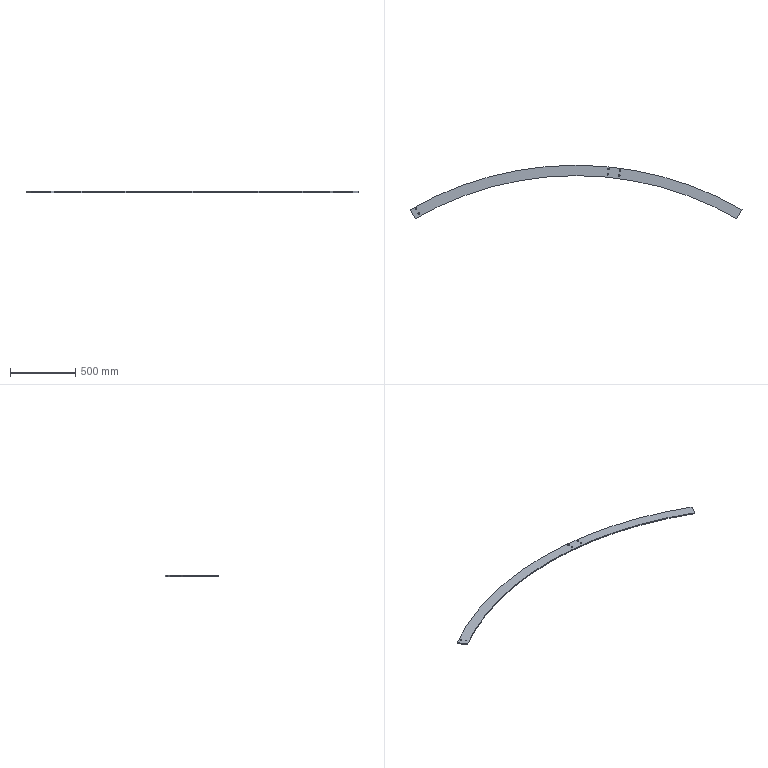Part | SolidWorks | features Extrusion 1, HoleWzd 1 | 1 solid | 18 faces | box 2550 x 410.917 x 8 mm | volume 1676789 mm3 | cylinder 14 | plane 4 | commonest cylinder face diameters 12 x12 4940 x1 5100 x1
STEP:
#1=CARTESIAN_POINT('',(-1221.329,76.713,0.));
#2=VERTEX_POINT('',#1);
#3=CARTESIAN_POINT('',(-1233.329,76.713,0.));
#4=VERTEX_POINT('',#3);
#5=CARTESIAN_POINT('',(-1227.329,76.713,0.));
#6=DIRECTION('',(0.,0.,-1.));
#7=DIRECTION('',(-1.,0.,0.));
#8=AXIS2_PLACEMENT_3D('',#5,#6,#7);
#9=CIRCLE('',#8,6.);
#10=EDGE_CURVE('',#2,#4,#9,.T.);
#11=ORIENTED_EDGE('',*,*,#10,.T.);
#12=CARTESIAN_POINT('',(-1233.329,76.713,8.));
#13=VERTEX_POINT('',#12);
#14=CARTESIAN_POINT('',(-1233.329,76.713,8.));
#15=DIRECTION('',(0.,0.,1.));
#16=VECTOR('',#15,1000.);
#17=LINE('',#14,#16);
#18=EDGE_CURVE('',#4,#13,#17,.T.);
#19=ORIENTED_EDGE('',*,*,#18,.T.);
#20=CARTESIAN_POINT('',(-1221.329,76.713,8.));
#21=VERTEX_POINT('',#20);
#22=CARTESIAN_POINT('',(-1227.329,76.713,8.));
#23=DIRECTION('',(0.,0.,1.));
#24=DIRECTION('',(1.,0.,0.));
#25=AXIS2_PLACEMENT_3D('',#22,#23,#24);
#26=CIRCLE('',#25,6.);
#27=EDGE_CURVE('',#13,#21,#26,.T.);
#28=ORIENTED_EDGE('',*,*,#27,.T.);
#29=CARTESIAN_POINT('',(-1221.329,76.713,8.));
#30=DIRECTION('',(0.,0.,1.));
#31=VECTOR('',#30,1000.);
#32=LINE('',#29,#31);
#33=EDGE_CURVE('',#2,#21,#32,.T.);
#34=ORIENTED_EDGE('',*,*,#33,.F.);
#35=EDGE_LOOP('',(#11,#19,#28,#34));
#36=FACE_OUTER_BOUND('',#35,.T.);
#37=CARTESIAN_POINT('',(-1227.329,76.713,8.));
#38=DIRECTION('',(0.,0.,1.));
#39=DIRECTION('',(1.,0.,0.));
#40=AXIS2_PLACEMENT_3D('',#37,#38,#39);
#41=CYLINDRICAL_SURFACE('',#40,6.);
#42=ADVANCED_FACE('',(#36),#41,.F.);
#43=CARTESIAN_POINT('',(-1201.948,41.723,0.));
#44=VERTEX_POINT('',#43);
#45=CARTESIAN_POINT('',(-1213.948,41.723,0.));
#46=VERTEX_POINT('',#45);
#47=CARTESIAN_POINT('',(-1207.948,41.723,0.));
#48=DIRECTION('',(0.,0.,-1.));
#49=DIRECTION('',(-1.,0.,0.));
#50=AXIS2_PLACEMENT_3D('',#47,#48,#49);
#51=CIRCLE('',#50,6.);
#52=EDGE_CURVE('',#44,#46,#51,.T.);
#53=ORIENTED_EDGE('',*,*,#52,.T.);
#54=CARTESIAN_POINT('',(-1213.948,41.723,8.));
#55=VERTEX_POINT('',#54);
#56=CARTESIAN_POINT('',(-1213.948,41.723,8.));
#57=DIRECTION('',(0.,0.,1.));
#58=VECTOR('',#57,1000.);
#59=LINE('',#56,#58);
#60=EDGE_CURVE('',#46,#55,#59,.T.);
#61=ORIENTED_EDGE('',*,*,#60,.T.);
#62=CARTESIAN_POINT('',(-1201.948,41.723,8.));
#63=VERTEX_POINT('',#62);
#64=CARTESIAN_POINT('',(-1207.948,41.723,8.));
#65=DIRECTION('',(0.,0.,1.));
#66=DIRECTION('',(1.,0.,0.));
#67=AXIS2_PLACEMENT_3D('',#64,#65,#66);
#68=CIRCLE('',#67,6.);
#69=EDGE_CURVE('',#55,#63,#68,.T.);
#70=ORIENTED_EDGE('',*,*,#69,.T.);
#71=CARTESIAN_POINT('',(-1201.948,41.723,8.));
#72=DIRECTION('',(0.,0.,1.));
#73=VECTOR('',#72,1000.);
#74=LINE('',#71,#73);
#75=EDGE_CURVE('',#44,#63,#74,.T.);
#76=ORIENTED_EDGE('',*,*,#75,.F.);
#77=EDGE_LOOP('',(#53,#61,#70,#76));
#78=FACE_OUTER_BOUND('',#77,.T.);
#79=CARTESIAN_POINT('',(-1207.948,41.723,8.));
#80=DIRECTION('',(0.,0.,1.));
#81=DIRECTION('',(1.,0.,0.));
#82=AXIS2_PLACEMENT_3D('',#79,#80,#81);
#83=CYLINDRICAL_SURFACE('',#82,6.);
#84=ADVANCED_FACE('',(#78),#83,.F.);
#85=CARTESIAN_POINT('',(254.497,381.698,0.));
#86=VERTEX_POINT('',#85);
#87=CARTESIAN_POINT('',(242.497,381.698,0.));
#88=VERTEX_POINT('',#87);
#89=CARTESIAN_POINT('',(248.497,381.698,0.));
#90=DIRECTION('',(0.,0.,-1.));
#91=DIRECTION('',(-1.,0.,0.));
#92=AXIS2_PLACEMENT_3D('',#89,#90,#91);
#93=CIRCLE('',#92,6.);
#94=EDGE_CURVE('',#86,#88,#93,.T.);
#95=ORIENTED_EDGE('',*,*,#94,.T.);
#96=CARTESIAN_POINT('',(242.497,381.698,8.));
#97=VERTEX_POINT('',#96);
#98=CARTESIAN_POINT('',(242.497,381.698,8.));
#99=DIRECTION('',(0.,0.,1.));
#100=VECTOR('',#99,1000.);
#101=LINE('',#98,#100);
#102=EDGE_CURVE('',#88,#97,#101,.T.);
#103=ORIENTED_EDGE('',*,*,#102,.T.);
#104=CARTESIAN_POINT('',(254.497,381.698,8.));
#105=VERTEX_POINT('',#104);
#106=CARTESIAN_POINT('',(248.497,381.698,8.));
#107=DIRECTION('',(0.,0.,1.));
#108=DIRECTION('',(1.,0.,0.));
#109=AXIS2_PLACEMENT_3D('',#106,#107,#108);
#110=CIRCLE('',#109,6.);
#111=EDGE_CURVE('',#97,#105,#110,.T.);
#112=ORIENTED_EDGE('',*,*,#111,.T.);
#113=CARTESIAN_POINT('',(254.497,381.698,8.));
#114=DIRECTION('',(0.,0.,1.));
#115=VECTOR('',#114,1000.);
#116=LINE('',#113,#115);
#117=EDGE_CURVE('',#86,#105,#116,.T.);
#118=ORIENTED_EDGE('',*,*,#117,.F.);
#119=EDGE_LOOP('',(#95,#103,#112,#118));
#120=FACE_OUTER_BOUND('',#119,.T.);
#121=CARTESIAN_POINT('',(248.497,381.698,8.));
#122=DIRECTION('',(0.,0.,1.));
#123=DIRECTION('',(1.,0.,0.));
#124=AXIS2_PLACEMENT_3D('',#121,#122,#123);
#125=CYLINDRICAL_SURFACE('',#124,6.);
#126=ADVANCED_FACE('',(#120),#125,.F.);
#127=CARTESIAN_POINT('',(250.573,341.891,0.));
#128=VERTEX_POINT('',#127);
#129=CARTESIAN_POINT('',(238.573,341.891,0.));
#130=VERTEX_POINT('',#129);
#131=CARTESIAN_POINT('',(244.573,341.891,0.));
#132=DIRECTION('',(0.,0.,-1.));
#133=DIRECTION('',(-1.,0.,0.));
#134=AXIS2_PLACEMENT_3D('',#131,#132,#133);
#135=CIRCLE('',#134,6.);
#136=EDGE_CURVE('',#128,#130,#135,.T.);
#137=ORIENTED_EDGE('',*,*,#136,.T.);
#138=CARTESIAN_POINT('',(238.573,341.891,8.));
#139=VERTEX_POINT('',#138);
#140=CARTESIAN_POINT('',(238.573,341.891,8.));
#141=DIRECTION('',(0.,0.,1.));
#142=VECTOR('',#141,1000.);
#143=LINE('',#140,#142);
#144=EDGE_CURVE('',#130,#139,#143,.T.);
#145=ORIENTED_EDGE('',*,*,#144,.T.);
#146=CARTESIAN_POINT('',(250.573,341.891,8.));
#147=VERTEX_POINT('',#146);
#148=CARTESIAN_POINT('',(244.573,341.891,8.));
#149=DIRECTION('',(0.,0.,1.));
#150=DIRECTION('',(1.,0.,0.));
#151=AXIS2_PLACEMENT_3D('',#148,#149,#150);
#152=CIRCLE('',#151,6.);
#153=EDGE_CURVE('',#139,#147,#152,.T.);
#154=ORIENTED_EDGE('',*,*,#153,.T.);
#155=CARTESIAN_POINT('',(250.573,341.891,8.));
#156=DIRECTION('',(0.,0.,1.));
#157=VECTOR('',#156,1000.);
#158=LINE('',#155,#157);
#159=EDGE_CURVE('',#128,#147,#158,.T.);
#160=ORIENTED_EDGE('',*,*,#159,.F.);
#161=EDGE_LOOP('',(#137,#145,#154,#160));
#162=FACE_OUTER_BOUND('',#161,.T.);
#163=CARTESIAN_POINT('',(244.573,341.891,8.));
#164=DIRECTION('',(0.,0.,1.));
#165=DIRECTION('',(1.,0.,0.));
#166=AXIS2_PLACEMENT_3D('',#163,#164,#165);
#167=CYLINDRICAL_SURFACE('',#166,6.);
#168=ADVANCED_FACE('',(#162),#167,.F.);
#169=CARTESIAN_POINT('',(343.892,371.279,0.));
#170=VERTEX_POINT('',#169);
#171=CARTESIAN_POINT('',(331.892,371.279,0.));
#172=VERTEX_POINT('',#171);
#173=CARTESIAN_POINT('',(337.892,371.279,0.));
#174=DIRECTION('',(0.,0.,-1.));
#175=DIRECTION('',(-1.,0.,0.));
#176=AXIS2_PLACEMENT_3D('',#173,#174,#175);
#177=CIRCLE('',#176,6.);
#178=EDGE_CURVE('',#170,#172,#177,.T.);
#179=ORIENTED_EDGE('',*,*,#178,.T.);
#180=CARTESIAN_POINT('',(331.892,371.279,8.));
#181=VERTEX_POINT('',#180);
#182=CARTESIAN_POINT('',(331.892,371.279,8.));
#183=DIRECTION('',(0.,0.,1.));
#184=VECTOR('',#183,1000.);
#185=LINE('',#182,#184);
#186=EDGE_CURVE('',#172,#181,#185,.T.);
#187=ORIENTED_EDGE('',*,*,#186,.T.);
#188=CARTESIAN_POINT('',(343.892,371.279,8.));
#189=VERTEX_POINT('',#188);
#190=CARTESIAN_POINT('',(337.892,371.279,8.));
#191=DIRECTION('',(0.,0.,1.));
#192=DIRECTION('',(1.,0.,0.));
#193=AXIS2_PLACEMENT_3D('',#190,#191,#192);
#194=CIRCLE('',#193,6.);
#195=EDGE_CURVE('',#181,#189,#194,.T.);
#196=ORIENTED_EDGE('',*,*,#195,.T.);
#197=CARTESIAN_POINT('',(343.892,371.279,8.));
#198=DIRECTION('',(0.,0.,1.));
#199=VECTOR('',#198,1000.);
#200=LINE('',#197,#199);
#201=EDGE_CURVE('',#170,#189,#200,.T.);
#202=ORIENTED_EDGE('',*,*,#201,.F.);
#203=EDGE_LOOP('',(#179,#187,#196,#202));
#204=FACE_OUTER_BOUND('',#203,.T.);
#205=CARTESIAN_POINT('',(337.892,371.279,8.));
#206=DIRECTION('',(0.,0.,1.));
#207=DIRECTION('',(1.,0.,0.));
#208=AXIS2_PLACEMENT_3D('',#205,#206,#207);
#209=CYLINDRICAL_SURFACE('',#208,6.);
#210=ADVANCED_FACE('',(#204),#209,.F.);
#211=CARTESIAN_POINT('',(338.556,331.637,0.));
#212=VERTEX_POINT('',#211);
#213=CARTESIAN_POINT('',(326.556,331.637,0.));
#214=VERTEX_POINT('',#213);
#215=CARTESIAN_POINT('',(332.556,331.637,0.));
#216=DIRECTION('',(0.,0.,-1.));
#217=DIRECTION('',(-1.,0.,0.));
#218=AXIS2_PLACEMENT_3D('',#215,#216,#217);
#219=CIRCLE('',#218,6.);
#220=EDGE_CURVE('',#212,#214,#219,.T.);
#221=ORIENTED_EDGE('',*,*,#220,.T.);
#222=CARTESIAN_POINT('',(326.556,331.637,8.));
#223=VERTEX_POINT('',#222);
#224=CARTESIAN_POINT('',(326.556,331.637,8.));
#225=DIRECTION('',(0.,0.,1.));
#226=VECTOR('',#225,1000.);
#227=LINE('',#224,#226);
#228=EDGE_CURVE('',#214,#223,#227,.T.);
#229=ORIENTED_EDGE('',*,*,#228,.T.);
#230=CARTESIAN_POINT('',(338.556,331.637,8.));
#231=VERTEX_POINT('',#230);
#232=CARTESIAN_POINT('',(332.556,331.637,8.));
#233=DIRECTION('',(0.,0.,1.));
#234=DIRECTION('',(1.,0.,0.));
#235=AXIS2_PLACEMENT_3D('',#232,#233,#234);
#236=CIRCLE('',#235,6.);
#237=EDGE_CURVE('',#223,#231,#236,.T.);
#238=ORIENTED_EDGE('',*,*,#237,.T.);
#239=CARTESIAN_POINT('',(338.556,331.637,8.));
#240=DIRECTION('',(0.,0.,1.));
#241=VECTOR('',#240,1000.);
#242=LINE('',#239,#241);
#243=EDGE_CURVE('',#212,#231,#242,.T.);
#244=ORIENTED_EDGE('',*,*,#243,.F.);
#245=EDGE_LOOP('',(#221,#229,#238,#244));
#246=FACE_OUTER_BOUND('',#245,.T.);
#247=CARTESIAN_POINT('',(332.556,331.637,8.));
#248=DIRECTION('',(0.,0.,1.));
#249=DIRECTION('',(1.,0.,0.));
#250=AXIS2_PLACEMENT_3D('',#247,#248,#249);
#251=CYLINDRICAL_SURFACE('',#250,6.);
#252=ADVANCED_FACE('',(#246),#251,.F.);
#253=CARTESIAN_POINT('',(-1207.948,41.723,8.));
#254=DIRECTION('',(0.,0.,1.));
#255=DIRECTION('',(1.,0.,0.));
#256=AXIS2_PLACEMENT_3D('',#253,#254,#255);
#257=CIRCLE('',#256,6.);
#258=EDGE_CURVE('',#63,#55,#257,.T.);
#259=ORIENTED_EDGE('',*,*,#258,.F.);
#260=ORIENTED_EDGE('',*,*,#69,.F.);
#261=EDGE_LOOP('',(#259,#260));
#262=FACE_BOUND('',#261,.T.);
#263=CARTESIAN_POINT('',(1275.,69.282,8.));
#264=VERTEX_POINT('',#263);
#265=CARTESIAN_POINT('',(-1275.,69.282,8.));
#266=VERTEX_POINT('',#265);
#267=CARTESIAN_POINT('',(0.,-2139.083,8.));
#268=DIRECTION('',(0.,0.,1.));
#269=DIRECTION('',(-1.,0.,0.));
#270=AXIS2_PLACEMENT_3D('',#267,#268,#269);
#271=CIRCLE('',#270,2550.);
#272=EDGE_CURVE('',#264,#266,#271,.T.);
#273=ORIENTED_EDGE('',*,*,#272,.T.);
#274=CARTESIAN_POINT('',(-1235.,0.,8.));
#275=VERTEX_POINT('',#274);
#276=CARTESIAN_POINT('',(-1275.,69.282,8.));
#277=DIRECTION('',(0.5,-0.866,0.));
#278=VECTOR('',#277,1000.);
#279=LINE('',#276,#278);
#280=EDGE_CURVE('',#266,#275,#279,.T.);
#281=ORIENTED_EDGE('',*,*,#280,.T.);
#282=CARTESIAN_POINT('',(1235.,0.,8.));
#283=VERTEX_POINT('',#282);
#284=CARTESIAN_POINT('',(0.,-2139.083,8.));
#285=DIRECTION('',(0.,0.,-1.));
#286=DIRECTION('',(-1.,0.,0.));
#287=AXIS2_PLACEMENT_3D('',#284,#285,#286);
#288=CIRCLE('',#287,2470.);
#289=EDGE_CURVE('',#275,#283,#288,.T.);
#290=ORIENTED_EDGE('',*,*,#289,.T.);
#291=CARTESIAN_POINT('',(1235.,0.,8.));
#292=DIRECTION('',(0.5,0.866,0.));
#293=VECTOR('',#292,1000.);
#294=LINE('',#291,#293);
#295=EDGE_CURVE('',#283,#264,#294,.T.);
#296=ORIENTED_EDGE('',*,*,#295,.T.);
#297=EDGE_LOOP('',(#273,#281,#290,#296));
#298=FACE_OUTER_BOUND('',#297,.T.);
#299=CARTESIAN_POINT('',(332.556,331.637,8.));
#300=DIRECTION('',(0.,0.,1.));
#301=DIRECTION('',(1.,0.,0.));
#302=AXIS2_PLACEMENT_3D('',#299,#300,#301);
#303=CIRCLE('',#302,6.);
#304=EDGE_CURVE('',#231,#223,#303,.T.);
#305=ORIENTED_EDGE('',*,*,#304,.F.);
#306=ORIENTED_EDGE('',*,*,#237,.F.);
#307=EDGE_LOOP('',(#305,#306));
#308=FACE_BOUND('',#307,.T.);
#309=CARTESIAN_POINT('',(337.892,371.279,8.));
#310=DIRECTION('',(0.,0.,1.));
#311=DIRECTION('',(1.,0.,0.));
#312=AXIS2_PLACEMENT_3D('',#309,#310,#311);
#313=CIRCLE('',#312,6.);
#314=EDGE_CURVE('',#189,#181,#313,.T.);
#315=ORIENTED_EDGE('',*,*,#314,.F.);
#316=ORIENTED_EDGE('',*,*,#195,.F.);
#317=EDGE_LOOP('',(#315,#316));
#318=FACE_BOUND('',#317,.T.);
#319=CARTESIAN_POINT('',(244.573,341.891,8.));
#320=DIRECTION('',(0.,0.,1.));
#321=DIRECTION('',(1.,0.,0.));
#322=AXIS2_PLACEMENT_3D('',#319,#320,#321);
#323=CIRCLE('',#322,6.);
#324=EDGE_CURVE('',#147,#139,#323,.T.);
#325=ORIENTED_EDGE('',*,*,#324,.F.);
#326=ORIENTED_EDGE('',*,*,#153,.F.);
#327=EDGE_LOOP('',(#325,#326));
#328=FACE_BOUND('',#327,.T.);
#329=CARTESIAN_POINT('',(248.497,381.698,8.));
#330=DIRECTION('',(0.,0.,1.));
#331=DIRECTION('',(1.,0.,0.));
#332=AXIS2_PLACEMENT_3D('',#329,#330,#331);
#333=CIRCLE('',#332,6.);
#334=EDGE_CURVE('',#105,#97,#333,.T.);
#335=ORIENTED_EDGE('',*,*,#334,.F.);
#336=ORIENTED_EDGE('',*,*,#111,.F.);
#337=EDGE_LOOP('',(#335,#336));
#338=FACE_BOUND('',#337,.T.);
#339=CARTESIAN_POINT('',(-1227.329,76.713,8.));
#340=DIRECTION('',(0.,0.,1.));
#341=DIRECTION('',(1.,0.,0.));
#342=AXIS2_PLACEMENT_3D('',#339,#340,#341);
#343=CIRCLE('',#342,6.);
#344=EDGE_CURVE('',#21,#13,#343,.T.);
#345=ORIENTED_EDGE('',*,*,#344,.F.);
#346=ORIENTED_EDGE('',*,*,#27,.F.);
#347=EDGE_LOOP('',(#345,#346));
#348=FACE_BOUND('',#347,.T.);
#349=CARTESIAN_POINT('',(0.,-2139.083,8.));
#350=DIRECTION('',(0.,0.,-1.));
#351=DIRECTION('',(-1.,0.,0.));
#352=AXIS2_PLACEMENT_3D('',#349,#350,#351);
#353=PLANE('',#352);
#354=ADVANCED_FACE('',(#262,#298,#308,#318,#328,#338,#348),#353,.F.);
#355=CARTESIAN_POINT('',(1275.,69.282,0.));
#356=VERTEX_POINT('',#355);
#357=CARTESIAN_POINT('',(-1275.,69.282,0.));
#358=VERTEX_POINT('',#357);
#359=CARTESIAN_POINT('',(0.,-2139.083,0.));
#360=DIRECTION('',(0.,0.,1.));
#361=DIRECTION('',(-1.,0.,0.));
#362=AXIS2_PLACEMENT_3D('',#359,#360,#361);
#363=CIRCLE('',#362,2550.);
#364=EDGE_CURVE('',#356,#358,#363,.T.);
#365=ORIENTED_EDGE('',*,*,#364,.T.);
#366=CARTESIAN_POINT('',(-1275.,69.282,8.));
#367=DIRECTION('',(0.,0.,-1.));
#368=VECTOR('',#367,1000.);
#369=LINE('',#366,#368);
#370=EDGE_CURVE('',#266,#358,#369,.T.);
#371=ORIENTED_EDGE('',*,*,#370,.F.);
#372=ORIENTED_EDGE('',*,*,#272,.F.);
#373=CARTESIAN_POINT('',(1275.,69.282,8.));
#374=DIRECTION('',(0.,0.,-1.));
#375=VECTOR('',#374,1000.);
#376=LINE('',#373,#375);
#377=EDGE_CURVE('',#264,#356,#376,.T.);
#378=ORIENTED_EDGE('',*,*,#377,.T.);
#379=EDGE_LOOP('',(#365,#371,#372,#378));
#380=FACE_OUTER_BOUND('',#379,.T.);
#381=CARTESIAN_POINT('',(0.,-2139.083,8.));
#382=DIRECTION('',(0.,0.,-1.));
#383=DIRECTION('',(-1.,0.,0.));
#384=AXIS2_PLACEMENT_3D('',#381,#382,#383);
#385=CYLINDRICAL_SURFACE('',#384,2550.);
#386=ADVANCED_FACE('',(#380),#385,.T.);
#387=CARTESIAN_POINT('',(-1235.,0.,0.));
#388=VERTEX_POINT('',#387);
#389=CARTESIAN_POINT('',(-1275.,69.282,0.));
#390=DIRECTION('',(0.5,-0.866,0.));
#391=VECTOR('',#390,1000.);
#392=LINE('',#389,#391);
#393=EDGE_CURVE('',#358,#388,#392,.T.);
#394=ORIENTED_EDGE('',*,*,#393,.T.);
#395=CARTESIAN_POINT('',(-1235.,0.,8.));
#396=DIRECTION('',(0.,0.,-1.));
#397=VECTOR('',#396,1000.);
#398=LINE('',#395,#397);
#399=EDGE_CURVE('',#275,#388,#398,.T.);
#400=ORIENTED_EDGE('',*,*,#399,.F.);
#401=ORIENTED_EDGE('',*,*,#280,.F.);
#402=ORIENTED_EDGE('',*,*,#370,.T.);
#403=EDGE_LOOP('',(#394,#400,#401,#402));
#404=FACE_OUTER_BOUND('',#403,.T.);
#405=CARTESIAN_POINT('',(-1275.,69.282,8.));
#406=DIRECTION('',(0.866,0.5,0.));
#407=DIRECTION('',(-0.5,0.866,0.));
#408=AXIS2_PLACEMENT_3D('',#405,#406,#407);
#409=PLANE('',#408);
#410=ADVANCED_FACE('',(#404),#409,.F.);
#411=CARTESIAN_POINT('',(1235.,0.,0.));
#412=VERTEX_POINT('',#411);
#413=CARTESIAN_POINT('',(0.,-2139.083,0.));
#414=DIRECTION('',(0.,0.,-1.));
#415=DIRECTION('',(-1.,0.,0.));
#416=AXIS2_PLACEMENT_3D('',#413,#414,#415);
#417=CIRCLE('',#416,2470.);
#418=EDGE_CURVE('',#388,#412,#417,.T.);
#419=ORIENTED_EDGE('',*,*,#418,.T.);
#420=CARTESIAN_POINT('',(1235.,0.,8.));
#421=DIRECTION('',(0.,0.,-1.));
#422=VECTOR('',#421,1000.);
#423=LINE('',#420,#422);
#424=EDGE_CURVE('',#283,#412,#423,.T.);
#425=ORIENTED_EDGE('',*,*,#424,.F.);
#426=ORIENTED_EDGE('',*,*,#289,.F.);
#427=ORIENTED_EDGE('',*,*,#399,.T.);
#428=EDGE_LOOP('',(#419,#425,#426,#427));
#429=FACE_OUTER_BOUND('',#428,.T.);
#430=CARTESIAN_POINT('',(0.,-2139.083,8.));
#431=DIRECTION('',(0.,0.,-1.));
#432=DIRECTION('',(-1.,0.,0.));
#433=AXIS2_PLACEMENT_3D('',#430,#431,#432);
#434=CYLINDRICAL_SURFACE('',#433,2470.);
#435=ADVANCED_FACE('',(#429),#434,.F.);
#436=CARTESIAN_POINT('',(1235.,0.,0.));
#437=DIRECTION('',(0.5,0.866,0.));
#438=VECTOR('',#437,1000.);
#439=LINE('',#436,#438);
#440=EDGE_CURVE('',#412,#356,#439,.T.);
#441=ORIENTED_EDGE('',*,*,#440,.T.);
#442=ORIENTED_EDGE('',*,*,#377,.F.);
#443=ORIENTED_EDGE('',*,*,#295,.F.);
#444=ORIENTED_EDGE('',*,*,#424,.T.);
#445=EDGE_LOOP('',(#441,#442,#443,#444));
#446=FACE_OUTER_BOUND('',#445,.T.);
#447=CARTESIAN_POINT('',(1235.,0.,8.));
#448=DIRECTION('',(-0.866,0.5,0.));
#449=DIRECTION('',(-0.5,-0.866,0.));
#450=AXIS2_PLACEMENT_3D('',#447,#448,#449);
#451=PLANE('',#450);
#452=ADVANCED_FACE('',(#446),#451,.F.);
#453=ORIENTED_EDGE('',*,*,#10,.F.);
#454=CARTESIAN_POINT('',(-1227.329,76.713,0.));
#455=DIRECTION('',(0.,0.,-1.));
#456=DIRECTION('',(-1.,0.,0.));
#457=AXIS2_PLACEMENT_3D('',#454,#455,#456);
#458=CIRCLE('',#457,6.);
#459=EDGE_CURVE('',#4,#2,#458,.T.);
#460=ORIENTED_EDGE('',*,*,#459,.F.);
#461=EDGE_LOOP('',(#453,#460));
#462=FACE_BOUND('',#461,.T.);
#463=ORIENTED_EDGE('',*,*,#52,.F.);
#464=CARTESIAN_POINT('',(-1207.948,41.723,0.));
#465=DIRECTION('',(0.,0.,-1.));
#466=DIRECTION('',(-1.,0.,0.));
#467=AXIS2_PLACEMENT_3D('',#464,#465,#466);
#468=CIRCLE('',#467,6.);
#469=EDGE_CURVE('',#46,#44,#468,.T.);
#470=ORIENTED_EDGE('',*,*,#469,.F.);
#471=EDGE_LOOP('',(#463,#470));
#472=FACE_BOUND('',#471,.T.);
#473=ORIENTED_EDGE('',*,*,#94,.F.);
#474=CARTESIAN_POINT('',(248.497,381.698,0.));
#475=DIRECTION('',(0.,0.,-1.));
#476=DIRECTION('',(-1.,0.,0.));
#477=AXIS2_PLACEMENT_3D('',#474,#475,#476);
#478=CIRCLE('',#477,6.);
#479=EDGE_CURVE('',#88,#86,#478,.T.);
#480=ORIENTED_EDGE('',*,*,#479,.F.);
#481=EDGE_LOOP('',(#473,#480));
#482=FACE_BOUND('',#481,.T.);
#483=ORIENTED_EDGE('',*,*,#136,.F.);
#484=CARTESIAN_POINT('',(244.573,341.891,0.));
#485=DIRECTION('',(0.,0.,-1.));
#486=DIRECTION('',(-1.,0.,0.));
#487=AXIS2_PLACEMENT_3D('',#484,#485,#486);
#488=CIRCLE('',#487,6.);
#489=EDGE_CURVE('',#130,#128,#488,.T.);
#490=ORIENTED_EDGE('',*,*,#489,.F.);
#491=EDGE_LOOP('',(#483,#490));
#492=FACE_BOUND('',#491,.T.);
#493=ORIENTED_EDGE('',*,*,#178,.F.);
#494=CARTESIAN_POINT('',(337.892,371.279,0.));
#495=DIRECTION('',(0.,0.,-1.));
#496=DIRECTION('',(-1.,0.,0.));
#497=AXIS2_PLACEMENT_3D('',#494,#495,#496);
#498=CIRCLE('',#497,6.);
#499=EDGE_CURVE('',#172,#170,#498,.T.);
#500=ORIENTED_EDGE('',*,*,#499,.F.);
#501=EDGE_LOOP('',(#493,#500));
#502=FACE_BOUND('',#501,.T.);
#503=ORIENTED_EDGE('',*,*,#220,.F.);
#504=CARTESIAN_POINT('',(332.556,331.637,0.));
#505=DIRECTION('',(0.,0.,-1.));
#506=DIRECTION('',(-1.,0.,0.));
#507=AXIS2_PLACEMENT_3D('',#504,#505,#506);
#508=CIRCLE('',#507,6.);
#509=EDGE_CURVE('',#214,#212,#508,.T.);
#510=ORIENTED_EDGE('',*,*,#509,.F.);
#511=EDGE_LOOP('',(#503,#510));
#512=FACE_BOUND('',#511,.T.);
#513=ORIENTED_EDGE('',*,*,#364,.F.);
#514=ORIENTED_EDGE('',*,*,#440,.F.);
#515=ORIENTED_EDGE('',*,*,#418,.F.);
#516=ORIENTED_EDGE('',*,*,#393,.F.);
#517=EDGE_LOOP('',(#513,#514,#515,#516));
#518=FACE_OUTER_BOUND('',#517,.T.);
#519=CARTESIAN_POINT('',(0.,-2139.083,0.));
#520=DIRECTION('',(0.,0.,-1.));
#521=DIRECTION('',(-1.,0.,0.));
#522=AXIS2_PLACEMENT_3D('',#519,#520,#521);
#523=PLANE('',#522);
#524=ADVANCED_FACE('',(#462,#472,#482,#492,#502,#512,#518),#523,.T.);
#525=ORIENTED_EDGE('',*,*,#228,.F.);
#526=ORIENTED_EDGE('',*,*,#509,.T.);
#527=ORIENTED_EDGE('',*,*,#243,.T.);
#528=ORIENTED_EDGE('',*,*,#304,.T.);
#529=EDGE_LOOP('',(#525,#526,#527,#528));
#530=FACE_OUTER_BOUND('',#529,.T.);
#531=CARTESIAN_POINT('',(332.556,331.637,8.));
#532=DIRECTION('',(0.,0.,1.));
#533=DIRECTION('',(1.,0.,0.));
#534=AXIS2_PLACEMENT_3D('',#531,#532,#533);
#535=CYLINDRICAL_SURFACE('',#534,6.);
#536=ADVANCED_FACE('',(#530),#535,.F.);
#537=ORIENTED_EDGE('',*,*,#186,.F.);
#538=ORIENTED_EDGE('',*,*,#499,.T.);
#539=ORIENTED_EDGE('',*,*,#201,.T.);
#540=ORIENTED_EDGE('',*,*,#314,.T.);
#541=EDGE_LOOP('',(#537,#538,#539,#540));
#542=FACE_OUTER_BOUND('',#541,.T.);
#543=CARTESIAN_POINT('',(337.892,371.279,8.));
#544=DIRECTION('',(0.,0.,1.));
#545=DIRECTION('',(1.,0.,0.));
#546=AXIS2_PLACEMENT_3D('',#543,#544,#545);
#547=CYLINDRICAL_SURFACE('',#546,6.);
#548=ADVANCED_FACE('',(#542),#547,.F.);
#549=ORIENTED_EDGE('',*,*,#144,.F.);
#550=ORIENTED_EDGE('',*,*,#489,.T.);
#551=ORIENTED_EDGE('',*,*,#159,.T.);
#552=ORIENTED_EDGE('',*,*,#324,.T.);
#553=EDGE_LOOP('',(#549,#550,#551,#552));
#554=FACE_OUTER_BOUND('',#553,.T.);
#555=CARTESIAN_POINT('',(244.573,341.891,8.));
#556=DIRECTION('',(0.,0.,1.));
#557=DIRECTION('',(1.,0.,0.));
#558=AXIS2_PLACEMENT_3D('',#555,#556,#557);
#559=CYLINDRICAL_SURFACE('',#558,6.);
#560=ADVANCED_FACE('',(#554),#559,.F.);
#561=ORIENTED_EDGE('',*,*,#102,.F.);
#562=ORIENTED_EDGE('',*,*,#479,.T.);
#563=ORIENTED_EDGE('',*,*,#117,.T.);
#564=ORIENTED_EDGE('',*,*,#334,.T.);
#565=EDGE_LOOP('',(#561,#562,#563,#564));
#566=FACE_OUTER_BOUND('',#565,.T.);
#567=CARTESIAN_POINT('',(248.497,381.698,8.));
#568=DIRECTION('',(0.,0.,1.));
#569=DIRECTION('',(1.,0.,0.));
#570=AXIS2_PLACEMENT_3D('',#567,#568,#569);
#571=CYLINDRICAL_SURFACE('',#570,6.);
#572=ADVANCED_FACE('',(#566),#571,.F.);
#573=ORIENTED_EDGE('',*,*,#60,.F.);
#574=ORIENTED_EDGE('',*,*,#469,.T.);
#575=ORIENTED_EDGE('',*,*,#75,.T.);
#576=ORIENTED_EDGE('',*,*,#258,.T.);
#577=EDGE_LOOP('',(#573,#574,#575,#576));
#578=FACE_OUTER_BOUND('',#577,.T.);
#579=CARTESIAN_POINT('',(-1207.948,41.723,8.));
#580=DIRECTION('',(0.,0.,1.));
#581=DIRECTION('',(1.,0.,0.));
#582=AXIS2_PLACEMENT_3D('',#579,#580,#581);
#583=CYLINDRICAL_SURFACE('',#582,6.);
#584=ADVANCED_FACE('',(#578),#583,.F.);
#585=ORIENTED_EDGE('',*,*,#18,.F.);
#586=ORIENTED_EDGE('',*,*,#459,.T.);
#587=ORIENTED_EDGE('',*,*,#33,.T.);
#588=ORIENTED_EDGE('',*,*,#344,.T.);
#589=EDGE_LOOP('',(#585,#586,#587,#588));
#590=FACE_OUTER_BOUND('',#589,.T.);
#591=CARTESIAN_POINT('',(-1227.329,76.713,8.));
#592=DIRECTION('',(0.,0.,1.));
#593=DIRECTION('',(1.,0.,0.));
#594=AXIS2_PLACEMENT_3D('',#591,#592,#593);
#595=CYLINDRICAL_SURFACE('',#594,6.);
#596=ADVANCED_FACE('',(#590),#595,.F.);
#597=CLOSED_SHELL('',(#42,#84,#126,#168,#210,#252,#354,#386,#410,#435,#452,#524,#536,#548,#560,#572,#584,#596));
#598=MANIFOLD_SOLID_BREP('',#597);
#599=CARTESIAN_POINT('',(0.,0.,0.));
#600=DIRECTION('',(0.,0.,1.));
#601=DIRECTION('',(1.,0.,0.));
#602=AXIS2_PLACEMENT_3D('',#599,#600,#601);
#603=(LENGTH_UNIT()NAMED_UNIT(*)SI_UNIT(.MILLI.,.METRE.));
#604=UNCERTAINTY_MEASURE_WITH_UNIT(LENGTH_MEASURE(0.00001),#603,'','');
#605=(NAMED_UNIT(*)PLANE_ANGLE_UNIT()SI_UNIT($,.RADIAN.));
#606=(NAMED_UNIT(*)SI_UNIT($,.STERADIAN.)SOLID_ANGLE_UNIT());
#607=(GEOMETRIC_REPRESENTATION_CONTEXT(3)GLOBAL_UNCERTAINTY_ASSIGNED_CONTEXT((#604))GLOBAL_UNIT_ASSIGNED_CONTEXT((#603,#605,#606))REPRESENTATION_CONTEXT('',''));
#608=ADVANCED_BREP_SHAPE_REPRESENTATION('',(#598,#602),#607);